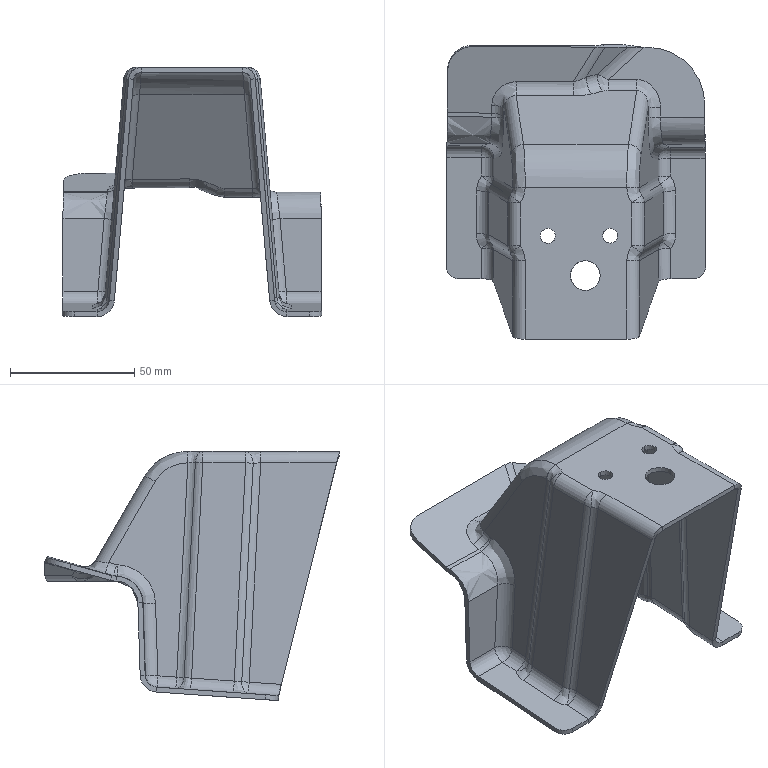Part | 1 solid | 193 faces | box 104.271 x 118.399 x 100.104 mm | volume 50929 mm3 | cylinder 79 | spline 70 | plane 23 | sphere 20 | other 1 | commonest cylinder face diameters 10 x32 14 x22 6 x16 18 x3 12 x2 22 x1